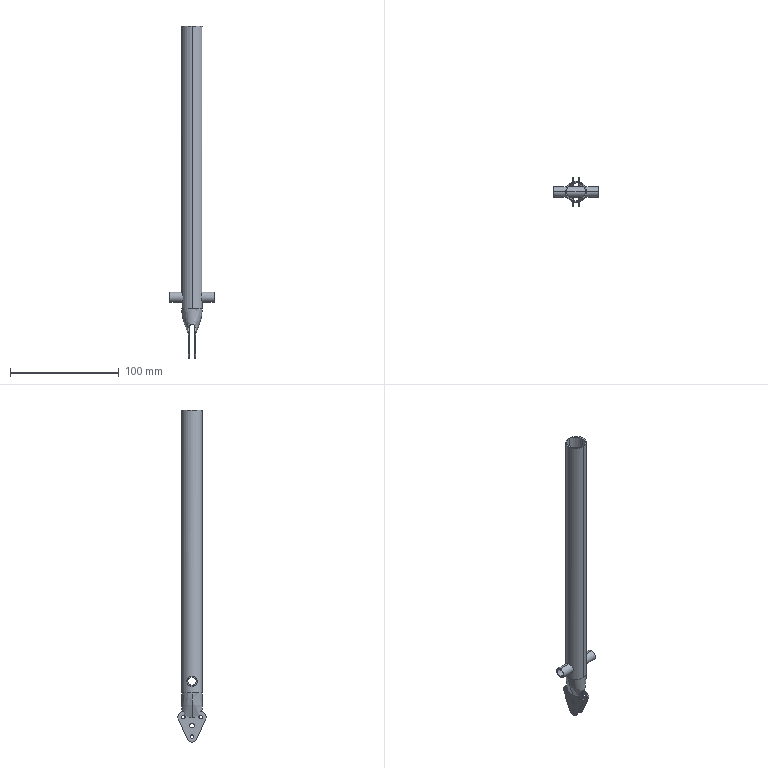Part | SolidWorks | features BaseBody 4 | 4 solids | 67 faces | box 41 x 26 x 306 mm | volume 15864 mm3 | cylinder 44 | plane 19 | spline 4 | commonest cylinder face diameters 3.175 x17 10 x7 9.525 x6 4.166 x4 5.08 x4 7.747 x2